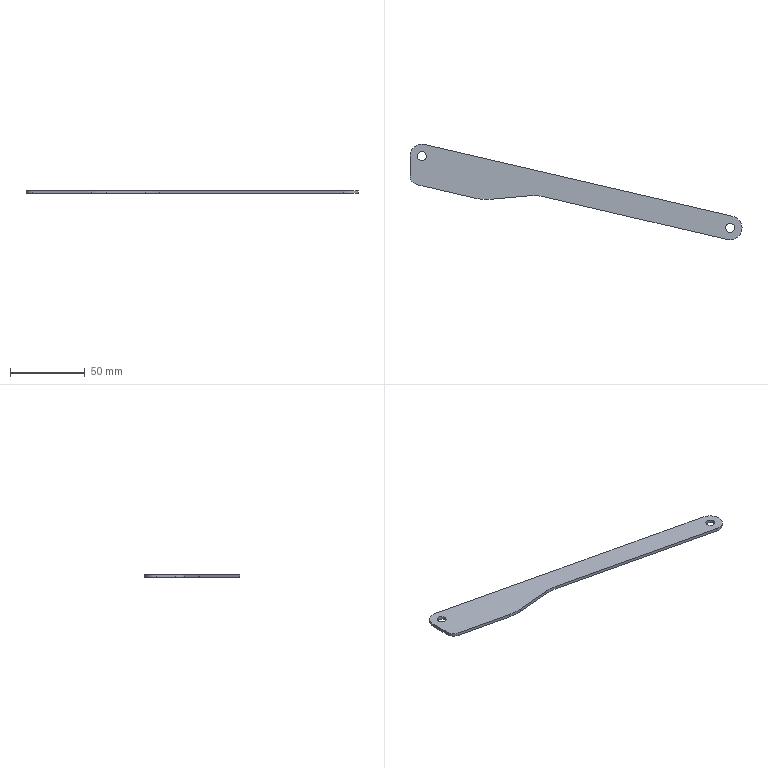Part | STEP file | 1 solid | 17 faces | box 222 x 64 x 2 mm | volume 8617 mm3 | cylinder 10 | plane 7 | commonest cylinder face diameters 6 x4 16 x3 60 x2 12 x1
STEP:
#1=CARTESIAN_POINT('',(0.,0.,0.));
#2=DIRECTION('',(0.,0.,1.));
#3=DIRECTION('',(1.,0.,0.));
#4=AXIS2_PLACEMENT_3D('',#1,#2,#3);
#5=CARTESIAN_POINT('',(115.253,-83.444,2.));
#6=VERTEX_POINT('',#5);
#7=CARTESIAN_POINT('',(125.069,-75.653,2.));
#8=VERTEX_POINT('',#7);
#9=CARTESIAN_POINT('',(117.069,-75.653,2.));
#10=DIRECTION('',(0.,0.,1.));
#11=DIRECTION('',(1.,0.,0.));
#12=AXIS2_PLACEMENT_3D('',#9,#10,#11);
#13=CIRCLE('',#12,8.);
#14=CARTESIAN_POINT('',(117.069,-75.653,2.));
#15=DIRECTION('',(0.,0.,1.));
#16=DIRECTION('',(1.,0.,0.));
#17=AXIS2_PLACEMENT_3D('',#14,#15,#16);
#18=CYLINDRICAL_SURFACE('',#17,8.);
#19=CARTESIAN_POINT('',(0.,0.));
#20=DIRECTION('',(1.,0.));
#21=VECTOR('',#20,1.);
#22=LINE('',#19,#21);
#23=(GEOMETRIC_REPRESENTATION_CONTEXT(2)PARAMETRIC_REPRESENTATION_CONTEXT()REPRESENTATION_CONTEXT('',''));
#24=DEFINITIONAL_REPRESENTATION('',(#22),#23);
#25=PCURVE('',#18,#24);
#26=CARTESIAN_POINT('',(11.579,-52.884,2.));
#27=DIRECTION('',(0.,0.,1.));
#28=DIRECTION('',(1.,0.,0.));
#29=AXIS2_PLACEMENT_3D('',#26,#27,#28);
#30=PLANE('',#29);
#31=CARTESIAN_POINT('',(105.49,-22.769));
#32=DIRECTION('',(1.,0.));
#33=AXIS2_PLACEMENT_2D('',#31,#32);
#34=CIRCLE('',#33,8.);
#35=(GEOMETRIC_REPRESENTATION_CONTEXT(2)PARAMETRIC_REPRESENTATION_CONTEXT()REPRESENTATION_CONTEXT('',''));
#36=DEFINITIONAL_REPRESENTATION('',(#34),#35);
#37=PCURVE('',#30,#36);
#38=SURFACE_CURVE('',#13,(#25,#37),.PCURVE_S1.);
#39=EDGE_CURVE('',#6,#8,#38,.T.);
#40=ORIENTED_EDGE('',*,*,#39,.T.);
#41=CARTESIAN_POINT('',(125.069,-75.653,4.));
#42=VERTEX_POINT('',#41);
#43=CARTESIAN_POINT('',(125.069,-75.653,2.));
#44=DIRECTION('',(0.,0.,1.));
#45=VECTOR('',#44,1.);
#46=LINE('',#43,#45);
#47=CARTESIAN_POINT('',(6.283,0.));
#48=DIRECTION('',(0.,1.));
#49=VECTOR('',#48,1.);
#50=LINE('',#47,#49);
#51=(GEOMETRIC_REPRESENTATION_CONTEXT(2)PARAMETRIC_REPRESENTATION_CONTEXT()REPRESENTATION_CONTEXT('',''));
#52=DEFINITIONAL_REPRESENTATION('',(#50),#51);
#53=PCURVE('',#18,#52);
#54=CARTESIAN_POINT('',(117.069,-75.653,2.));
#55=DIRECTION('',(0.,0.,1.));
#56=DIRECTION('',(1.,0.,0.));
#57=AXIS2_PLACEMENT_3D('',#54,#55,#56);
#58=CYLINDRICAL_SURFACE('',#57,8.);
#59=CARTESIAN_POINT('',(0.,0.));
#60=DIRECTION('',(0.,1.));
#61=VECTOR('',#60,1.);
#62=LINE('',#59,#61);
#63=(GEOMETRIC_REPRESENTATION_CONTEXT(2)PARAMETRIC_REPRESENTATION_CONTEXT()REPRESENTATION_CONTEXT('',''));
#64=DEFINITIONAL_REPRESENTATION('',(#62),#63);
#65=PCURVE('',#58,#64);
#66=SURFACE_CURVE('',#46,(#53,#65),.PCURVE_S1.);
#67=EDGE_CURVE('',#8,#42,#66,.T.);
#68=ORIENTED_EDGE('',*,*,#67,.T.);
#69=CARTESIAN_POINT('',(115.253,-83.444,4.));
#70=VERTEX_POINT('',#69);
#71=CARTESIAN_POINT('',(117.069,-75.653,4.));
#72=DIRECTION('',(0.,0.,-1.));
#73=DIRECTION('',(1.,0.,0.));
#74=AXIS2_PLACEMENT_3D('',#71,#72,#73);
#75=CIRCLE('',#74,8.);
#76=CARTESIAN_POINT('',(6.283,2.));
#77=DIRECTION('',(-1.,0.));
#78=VECTOR('',#77,1.);
#79=LINE('',#76,#78);
#80=(GEOMETRIC_REPRESENTATION_CONTEXT(2)PARAMETRIC_REPRESENTATION_CONTEXT()REPRESENTATION_CONTEXT('',''));
#81=DEFINITIONAL_REPRESENTATION('',(#79),#80);
#82=PCURVE('',#18,#81);
#83=CARTESIAN_POINT('',(11.579,-52.884,4.));
#84=DIRECTION('',(0.,0.,1.));
#85=DIRECTION('',(1.,0.,0.));
#86=AXIS2_PLACEMENT_3D('',#83,#84,#85);
#87=PLANE('',#86);
#88=CARTESIAN_POINT('',(113.49,-22.769));
#89=CARTESIAN_POINT('',(113.49,-36.625));
#90=CARTESIAN_POINT('',(101.49,-29.697));
#91=CARTESIAN_POINT('',(89.49,-22.769));
#92=CARTESIAN_POINT('',(101.49,-15.841));
#93=CARTESIAN_POINT('',(113.49,-8.912));
#94=CARTESIAN_POINT('',(113.49,-22.769));
#95=(BOUNDED_CURVE()B_SPLINE_CURVE(2,(#88,#89,#90,#91,#92,#93,#94),.UNSPECIFIED.,.T.,.F.)B_SPLINE_CURVE_WITH_KNOTS((1,2,2,2,2,1),(-2.094,0.,2.094,4.189,6.283,8.378),.UNSPECIFIED.)CURVE()GEOMETRIC_REPRESENTATION_ITEM()RATIONAL_B_SPLINE_CURVE((1.,0.5,1.,0.5,1.,0.5,1.))REPRESENTATION_ITEM(''));
#96=(GEOMETRIC_REPRESENTATION_CONTEXT(2)PARAMETRIC_REPRESENTATION_CONTEXT()REPRESENTATION_CONTEXT('',''));
#97=DEFINITIONAL_REPRESENTATION('',(#95),#96);
#98=PCURVE('',#87,#97);
#99=SURFACE_CURVE('',#75,(#82,#98),.PCURVE_S1.);
#100=EDGE_CURVE('',#42,#70,#99,.T.);
#101=ORIENTED_EDGE('',*,*,#100,.T.);
#102=CARTESIAN_POINT('',(115.253,-83.444,2.));
#103=DIRECTION('',(0.,0.,-1.));
#104=VECTOR('',#103,1.);
#105=LINE('',#102,#104);
#106=CARTESIAN_POINT('',(4.483,0.));
#107=DIRECTION('',(0.,-1.));
#108=VECTOR('',#107,1.);
#109=LINE('',#106,#108);
#110=(GEOMETRIC_REPRESENTATION_CONTEXT(2)PARAMETRIC_REPRESENTATION_CONTEXT()REPRESENTATION_CONTEXT('',''));
#111=DEFINITIONAL_REPRESENTATION('',(#109),#110);
#112=PCURVE('',#18,#111);
#113=CARTESIAN_POINT('',(-7.662,-54.804,2.));
#114=DIRECTION('',(-0.2269,-0.9739,0.));
#115=DIRECTION('',(0.9739,-0.2269,0.));
#116=AXIS2_PLACEMENT_3D('',#113,#114,#115);
#117=PLANE('',#116);
#118=CARTESIAN_POINT('',(126.208,0.));
#119=DIRECTION('',(0.,-1.));
#120=VECTOR('',#119,1.);
#121=LINE('',#118,#120);
#122=(GEOMETRIC_REPRESENTATION_CONTEXT(2)PARAMETRIC_REPRESENTATION_CONTEXT()REPRESENTATION_CONTEXT('',''));
#123=DEFINITIONAL_REPRESENTATION('',(#121),#122);
#124=PCURVE('',#117,#123);
#125=SURFACE_CURVE('',#105,(#112,#124),.PCURVE_S1.);
#126=EDGE_CURVE('',#70,#6,#125,.T.);
#127=ORIENTED_EDGE('',*,*,#126,.T.);
#128=EDGE_LOOP('',(#40,#68,#101,#127));
#129=FACE_BOUND('',#128,.T.);
#130=ADVANCED_FACE('',(#129),#18,.T.);
#131=CARTESIAN_POINT('',(120.069,-75.653,2.));
#132=VERTEX_POINT('',#131);
#133=CARTESIAN_POINT('',(120.069,-75.653,4.));
#134=VERTEX_POINT('',#133);
#135=CARTESIAN_POINT('',(120.069,-75.653,2.));
#136=DIRECTION('',(0.,0.,1.));
#137=VECTOR('',#136,1.);
#138=LINE('',#135,#137);
#139=CARTESIAN_POINT('',(117.069,-75.653,2.));
#140=DIRECTION('',(0.,0.,1.));
#141=DIRECTION('',(1.,0.,0.));
#142=AXIS2_PLACEMENT_3D('',#139,#140,#141);
#143=CYLINDRICAL_SURFACE('',#142,3.);
#144=CARTESIAN_POINT('',(6.283,0.));
#145=DIRECTION('',(0.,1.));
#146=VECTOR('',#145,1.);
#147=LINE('',#144,#146);
#148=(GEOMETRIC_REPRESENTATION_CONTEXT(2)PARAMETRIC_REPRESENTATION_CONTEXT()REPRESENTATION_CONTEXT('',''));
#149=DEFINITIONAL_REPRESENTATION('',(#147),#148);
#150=PCURVE('',#143,#149);
#151=CARTESIAN_POINT('',(117.069,-75.653,2.));
#152=DIRECTION('',(0.,0.,1.));
#153=DIRECTION('',(1.,0.,0.));
#154=AXIS2_PLACEMENT_3D('',#151,#152,#153);
#155=CYLINDRICAL_SURFACE('',#154,3.);
#156=CARTESIAN_POINT('',(0.,0.));
#157=DIRECTION('',(0.,1.));
#158=VECTOR('',#157,1.);
#159=LINE('',#156,#158);
#160=(GEOMETRIC_REPRESENTATION_CONTEXT(2)PARAMETRIC_REPRESENTATION_CONTEXT()REPRESENTATION_CONTEXT('',''));
#161=DEFINITIONAL_REPRESENTATION('',(#159),#160);
#162=PCURVE('',#155,#161);
#163=SURFACE_CURVE('',#138,(#150,#162),.PCURVE_S1.);
#164=EDGE_CURVE('',#132,#134,#163,.T.);
#165=ORIENTED_EDGE('',*,*,#164,.T.);
#166=CARTESIAN_POINT('',(114.069,-75.653,4.));
#167=VERTEX_POINT('',#166);
#168=CARTESIAN_POINT('',(117.069,-75.653,4.));
#169=DIRECTION('',(0.,0.,-1.));
#170=DIRECTION('',(1.,0.,0.));
#171=AXIS2_PLACEMENT_3D('',#168,#169,#170);
#172=CIRCLE('',#171,3.);
#173=CARTESIAN_POINT('',(6.283,2.));
#174=DIRECTION('',(-1.,0.));
#175=VECTOR('',#174,1.);
#176=LINE('',#173,#175);
#177=(GEOMETRIC_REPRESENTATION_CONTEXT(2)PARAMETRIC_REPRESENTATION_CONTEXT()REPRESENTATION_CONTEXT('',''));
#178=DEFINITIONAL_REPRESENTATION('',(#176),#177);
#179=PCURVE('',#143,#178);
#180=CARTESIAN_POINT('',(108.49,-22.769));
#181=CARTESIAN_POINT('',(108.49,-27.965));
#182=CARTESIAN_POINT('',(103.99,-25.367));
#183=CARTESIAN_POINT('',(99.49,-22.769));
#184=CARTESIAN_POINT('',(103.99,-20.171));
#185=CARTESIAN_POINT('',(108.49,-17.573));
#186=CARTESIAN_POINT('',(108.49,-22.769));
#187=(BOUNDED_CURVE()B_SPLINE_CURVE(2,(#180,#181,#182,#183,#184,#185,#186),.UNSPECIFIED.,.T.,.F.)B_SPLINE_CURVE_WITH_KNOTS((1,2,2,2,2,1),(-2.094,0.,2.094,4.189,6.283,8.378),.UNSPECIFIED.)CURVE()GEOMETRIC_REPRESENTATION_ITEM()RATIONAL_B_SPLINE_CURVE((1.,0.5,1.,0.5,1.,0.5,1.))REPRESENTATION_ITEM(''));
#188=(GEOMETRIC_REPRESENTATION_CONTEXT(2)PARAMETRIC_REPRESENTATION_CONTEXT()REPRESENTATION_CONTEXT('',''));
#189=DEFINITIONAL_REPRESENTATION('',(#187),#188);
#190=PCURVE('',#87,#189);
#191=SURFACE_CURVE('',#172,(#179,#190),.PCURVE_S1.);
#192=EDGE_CURVE('',#134,#167,#191,.T.);
#193=ORIENTED_EDGE('',*,*,#192,.T.);
#194=CARTESIAN_POINT('',(114.069,-75.653,2.));
#195=VERTEX_POINT('',#194);
#196=CARTESIAN_POINT('',(114.069,-75.653,2.));
#197=DIRECTION('',(0.,0.,1.));
#198=VECTOR('',#197,1.);
#199=LINE('',#196,#198);
#200=CARTESIAN_POINT('',(3.142,0.));
#201=DIRECTION('',(0.,1.));
#202=VECTOR('',#201,1.);
#203=LINE('',#200,#202);
#204=(GEOMETRIC_REPRESENTATION_CONTEXT(2)PARAMETRIC_REPRESENTATION_CONTEXT()REPRESENTATION_CONTEXT('',''));
#205=DEFINITIONAL_REPRESENTATION('',(#203),#204);
#206=PCURVE('',#143,#205);
#207=CARTESIAN_POINT('',(3.142,0.));
#208=DIRECTION('',(0.,1.));
#209=VECTOR('',#208,1.);
#210=LINE('',#207,#209);
#211=(GEOMETRIC_REPRESENTATION_CONTEXT(2)PARAMETRIC_REPRESENTATION_CONTEXT()REPRESENTATION_CONTEXT('',''));
#212=DEFINITIONAL_REPRESENTATION('',(#210),#211);
#213=PCURVE('',#155,#212);
#214=SURFACE_CURVE('',#199,(#206,#213),.PCURVE_S1.);
#215=EDGE_CURVE('',#195,#167,#214,.T.);
#216=ORIENTED_EDGE('',*,*,#215,.F.);
#217=CARTESIAN_POINT('',(117.069,-75.653,2.));
#218=DIRECTION('',(0.,0.,-1.));
#219=DIRECTION('',(1.,0.,0.));
#220=AXIS2_PLACEMENT_3D('',#217,#218,#219);
#221=CIRCLE('',#220,3.);
#222=CARTESIAN_POINT('',(6.283,0.));
#223=DIRECTION('',(-1.,0.));
#224=VECTOR('',#223,1.);
#225=LINE('',#222,#224);
#226=(GEOMETRIC_REPRESENTATION_CONTEXT(2)PARAMETRIC_REPRESENTATION_CONTEXT()REPRESENTATION_CONTEXT('',''));
#227=DEFINITIONAL_REPRESENTATION('',(#225),#226);
#228=PCURVE('',#143,#227);
#229=CARTESIAN_POINT('',(108.49,-22.769));
#230=CARTESIAN_POINT('',(108.49,-27.965));
#231=CARTESIAN_POINT('',(103.99,-25.367));
#232=CARTESIAN_POINT('',(99.49,-22.769));
#233=CARTESIAN_POINT('',(103.99,-20.171));
#234=CARTESIAN_POINT('',(108.49,-17.573));
#235=CARTESIAN_POINT('',(108.49,-22.769));
#236=(BOUNDED_CURVE()B_SPLINE_CURVE(2,(#229,#230,#231,#232,#233,#234,#235),.UNSPECIFIED.,.T.,.F.)B_SPLINE_CURVE_WITH_KNOTS((1,2,2,2,2,1),(-2.094,0.,2.094,4.189,6.283,8.378),.UNSPECIFIED.)CURVE()GEOMETRIC_REPRESENTATION_ITEM()RATIONAL_B_SPLINE_CURVE((1.,0.5,1.,0.5,1.,0.5,1.))REPRESENTATION_ITEM(''));
#237=(GEOMETRIC_REPRESENTATION_CONTEXT(2)PARAMETRIC_REPRESENTATION_CONTEXT()REPRESENTATION_CONTEXT('',''));
#238=DEFINITIONAL_REPRESENTATION('',(#236),#237);
#239=PCURVE('',#30,#238);
#240=SURFACE_CURVE('',#221,(#228,#239),.PCURVE_S1.);
#241=EDGE_CURVE('',#132,#195,#240,.T.);
#242=ORIENTED_EDGE('',*,*,#241,.F.);
#243=EDGE_LOOP('',(#165,#193,#216,#242));
#244=FACE_BOUND('',#243,.F.);
#245=ADVANCED_FACE('',(#244),#143,.F.);
#246=CARTESIAN_POINT('',(-85.931,-27.653,2.));
#247=VERTEX_POINT('',#246);
#248=CARTESIAN_POINT('',(-85.931,-27.653,4.));
#249=VERTEX_POINT('',#248);
#250=CARTESIAN_POINT('',(-85.931,-27.653,2.));
#251=DIRECTION('',(0.,0.,1.));
#252=VECTOR('',#251,1.);
#253=LINE('',#250,#252);
#254=CARTESIAN_POINT('',(-88.931,-27.653,2.));
#255=DIRECTION('',(0.,0.,1.));
#256=DIRECTION('',(1.,0.,0.));
#257=AXIS2_PLACEMENT_3D('',#254,#255,#256);
#258=CYLINDRICAL_SURFACE('',#257,3.);
#259=CARTESIAN_POINT('',(6.283,0.));
#260=DIRECTION('',(0.,1.));
#261=VECTOR('',#260,1.);
#262=LINE('',#259,#261);
#263=(GEOMETRIC_REPRESENTATION_CONTEXT(2)PARAMETRIC_REPRESENTATION_CONTEXT()REPRESENTATION_CONTEXT('',''));
#264=DEFINITIONAL_REPRESENTATION('',(#262),#263);
#265=PCURVE('',#258,#264);
#266=CARTESIAN_POINT('',(-88.931,-27.653,2.));
#267=DIRECTION('',(0.,0.,1.));
#268=DIRECTION('',(1.,0.,0.));
#269=AXIS2_PLACEMENT_3D('',#266,#267,#268);
#270=CYLINDRICAL_SURFACE('',#269,3.);
#271=CARTESIAN_POINT('',(0.,0.));
#272=DIRECTION('',(0.,1.));
#273=VECTOR('',#272,1.);
#274=LINE('',#271,#273);
#275=(GEOMETRIC_REPRESENTATION_CONTEXT(2)PARAMETRIC_REPRESENTATION_CONTEXT()REPRESENTATION_CONTEXT('',''));
#276=DEFINITIONAL_REPRESENTATION('',(#274),#275);
#277=PCURVE('',#270,#276);
#278=SURFACE_CURVE('',#253,(#265,#277),.PCURVE_S1.);
#279=EDGE_CURVE('',#247,#249,#278,.T.);
#280=ORIENTED_EDGE('',*,*,#279,.T.);
#281=CARTESIAN_POINT('',(-91.931,-27.653,4.));
#282=VERTEX_POINT('',#281);
#283=CARTESIAN_POINT('',(-88.931,-27.653,4.));
#284=DIRECTION('',(0.,0.,-1.));
#285=DIRECTION('',(1.,0.,0.));
#286=AXIS2_PLACEMENT_3D('',#283,#284,#285);
#287=CIRCLE('',#286,3.);
#288=CARTESIAN_POINT('',(6.283,2.));
#289=DIRECTION('',(-1.,0.));
#290=VECTOR('',#289,1.);
#291=LINE('',#288,#290);
#292=(GEOMETRIC_REPRESENTATION_CONTEXT(2)PARAMETRIC_REPRESENTATION_CONTEXT()REPRESENTATION_CONTEXT('',''));
#293=DEFINITIONAL_REPRESENTATION('',(#291),#292);
#294=PCURVE('',#258,#293);
#295=CARTESIAN_POINT('',(-97.51,25.231));
#296=CARTESIAN_POINT('',(-97.51,20.035));
#297=CARTESIAN_POINT('',(-102.01,22.633));
#298=CARTESIAN_POINT('',(-106.51,25.231));
#299=CARTESIAN_POINT('',(-102.01,27.829));
#300=CARTESIAN_POINT('',(-97.51,30.427));
#301=CARTESIAN_POINT('',(-97.51,25.231));
#302=(BOUNDED_CURVE()B_SPLINE_CURVE(2,(#295,#296,#297,#298,#299,#300,#301),.UNSPECIFIED.,.T.,.F.)B_SPLINE_CURVE_WITH_KNOTS((1,2,2,2,2,1),(-2.094,0.,2.094,4.189,6.283,8.378),.UNSPECIFIED.)CURVE()GEOMETRIC_REPRESENTATION_ITEM()RATIONAL_B_SPLINE_CURVE((1.,0.5,1.,0.5,1.,0.5,1.))REPRESENTATION_ITEM(''));
#303=(GEOMETRIC_REPRESENTATION_CONTEXT(2)PARAMETRIC_REPRESENTATION_CONTEXT()REPRESENTATION_CONTEXT('',''));
#304=DEFINITIONAL_REPRESENTATION('',(#302),#303);
#305=PCURVE('',#87,#304);
#306=SURFACE_CURVE('',#287,(#294,#305),.PCURVE_S1.);
#307=EDGE_CURVE('',#249,#282,#306,.T.);
#308=ORIENTED_EDGE('',*,*,#307,.T.);
#309=CARTESIAN_POINT('',(-91.931,-27.653,2.));
#310=VERTEX_POINT('',#309);
#311=CARTESIAN_POINT('',(-91.931,-27.653,2.));
#312=DIRECTION('',(0.,0.,1.));
#313=VECTOR('',#312,1.);
#314=LINE('',#311,#313);
#315=CARTESIAN_POINT('',(3.142,0.));
#316=DIRECTION('',(0.,1.));
#317=VECTOR('',#316,1.);
#318=LINE('',#315,#317);
#319=(GEOMETRIC_REPRESENTATION_CONTEXT(2)PARAMETRIC_REPRESENTATION_CONTEXT()REPRESENTATION_CONTEXT('',''));
#320=DEFINITIONAL_REPRESENTATION('',(#318),#319);
#321=PCURVE('',#258,#320);
#322=CARTESIAN_POINT('',(3.142,0.));
#323=DIRECTION('',(0.,1.));
#324=VECTOR('',#323,1.);
#325=LINE('',#322,#324);
#326=(GEOMETRIC_REPRESENTATION_CONTEXT(2)PARAMETRIC_REPRESENTATION_CONTEXT()REPRESENTATION_CONTEXT('',''));
#327=DEFINITIONAL_REPRESENTATION('',(#325),#326);
#328=PCURVE('',#270,#327);
#329=SURFACE_CURVE('',#314,(#321,#328),.PCURVE_S1.);
#330=EDGE_CURVE('',#310,#282,#329,.T.);
#331=ORIENTED_EDGE('',*,*,#330,.F.);
#332=CARTESIAN_POINT('',(-88.931,-27.653,2.));
#333=DIRECTION('',(0.,0.,-1.));
#334=DIRECTION('',(1.,0.,0.));
#335=AXIS2_PLACEMENT_3D('',#332,#333,#334);
#336=CIRCLE('',#335,3.);
#337=CARTESIAN_POINT('',(6.283,0.));
#338=DIRECTION('',(-1.,0.));
#339=VECTOR('',#338,1.);
#340=LINE('',#337,#339);
#341=(GEOMETRIC_REPRESENTATION_CONTEXT(2)PARAMETRIC_REPRESENTATION_CONTEXT()REPRESENTATION_CONTEXT('',''));
#342=DEFINITIONAL_REPRESENTATION('',(#340),#341);
#343=PCURVE('',#258,#342);
#344=CARTESIAN_POINT('',(-97.51,25.231));
#345=CARTESIAN_POINT('',(-97.51,20.035));
#346=CARTESIAN_POINT('',(-102.01,22.633));
#347=CARTESIAN_POINT('',(-106.51,25.231));
#348=CARTESIAN_POINT('',(-102.01,27.829));
#349=CARTESIAN_POINT('',(-97.51,30.427));
#350=CARTESIAN_POINT('',(-97.51,25.231));
#351=(BOUNDED_CURVE()B_SPLINE_CURVE(2,(#344,#345,#346,#347,#348,#349,#350),.UNSPECIFIED.,.T.,.F.)B_SPLINE_CURVE_WITH_KNOTS((1,2,2,2,2,1),(-2.094,0.,2.094,4.189,6.283,8.378),.UNSPECIFIED.)CURVE()GEOMETRIC_REPRESENTATION_ITEM()RATIONAL_B_SPLINE_CURVE((1.,0.5,1.,0.5,1.,0.5,1.))REPRESENTATION_ITEM(''));
#352=(GEOMETRIC_REPRESENTATION_CONTEXT(2)PARAMETRIC_REPRESENTATION_CONTEXT()REPRESENTATION_CONTEXT('',''));
#353=DEFINITIONAL_REPRESENTATION('',(#351),#352);
#354=PCURVE('',#30,#353);
#355=SURFACE_CURVE('',#336,(#343,#354),.PCURVE_S1.);
#356=EDGE_CURVE('',#247,#310,#355,.T.);
#357=ORIENTED_EDGE('',*,*,#356,.F.);
#358=EDGE_LOOP('',(#280,#308,#331,#357));
#359=FACE_BOUND('',#358,.F.);
#360=ADVANCED_FACE('',(#359),#258,.F.);
#361=ORIENTED_EDGE('',*,*,#39,.F.);
#362=CARTESIAN_POINT('',(-7.662,-54.804,2.));
#363=VERTEX_POINT('',#362);
#364=CARTESIAN_POINT('',(-7.662,-54.804,2.));
#365=DIRECTION('',(0.9739,-0.2269,0.));
#366=VECTOR('',#365,1.);
#367=LINE('',#364,#366);
#368=CARTESIAN_POINT('',(-19.242,-1.919));
#369=DIRECTION('',(0.9739,-0.2269));
#370=VECTOR('',#369,1.);
#371=LINE('',#368,#370);
#372=(GEOMETRIC_REPRESENTATION_CONTEXT(2)PARAMETRIC_REPRESENTATION_CONTEXT()REPRESENTATION_CONTEXT('',''));
#373=DEFINITIONAL_REPRESENTATION('',(#371),#372);
#374=PCURVE('',#30,#373);
#375=CARTESIAN_POINT('',(0.,0.));
#376=DIRECTION('',(1.,0.));
#377=VECTOR('',#376,1.);
#378=LINE('',#375,#377);
#379=(GEOMETRIC_REPRESENTATION_CONTEXT(2)PARAMETRIC_REPRESENTATION_CONTEXT()REPRESENTATION_CONTEXT('',''));
#380=DEFINITIONAL_REPRESENTATION('',(#378),#379);
#381=PCURVE('',#117,#380);
#382=SURFACE_CURVE('',#367,(#374,#381),.PCURVE_S1.);
#383=EDGE_CURVE('',#363,#6,#382,.T.);
#384=ORIENTED_EDGE('',*,*,#383,.F.);
#385=CARTESIAN_POINT('',(-17.217,-54.147,2.));
#386=VERTEX_POINT('',#385);
#387=CARTESIAN_POINT('',(-14.47,-84.021,2.));
#388=DIRECTION('',(0.,0.,-1.));
#389=DIRECTION('',(1.,0.,0.));
#390=AXIS2_PLACEMENT_3D('',#387,#388,#389);
#391=CIRCLE('',#390,30.);
#392=CARTESIAN_POINT('',(3.95,-31.137));
#393=CARTESIAN_POINT('',(3.95,-83.098));
#394=CARTESIAN_POINT('',(-41.05,-57.118));
#395=CARTESIAN_POINT('',(-86.05,-31.137));
#396=CARTESIAN_POINT('',(-41.05,-5.156));
#397=CARTESIAN_POINT('',(3.95,20.825));
#398=CARTESIAN_POINT('',(3.95,-31.137));
#399=(BOUNDED_CURVE()B_SPLINE_CURVE(2,(#392,#393,#394,#395,#396,#397,#398),.UNSPECIFIED.,.T.,.F.)B_SPLINE_CURVE_WITH_KNOTS((1,2,2,2,2,1),(-2.094,0.,2.094,4.189,6.283,8.378),.UNSPECIFIED.)CURVE()GEOMETRIC_REPRESENTATION_ITEM()RATIONAL_B_SPLINE_CURVE((1.,0.5,1.,0.5,1.,0.5,1.))REPRESENTATION_ITEM(''));
#400=(GEOMETRIC_REPRESENTATION_CONTEXT(2)PARAMETRIC_REPRESENTATION_CONTEXT()REPRESENTATION_CONTEXT('',''));
#401=DEFINITIONAL_REPRESENTATION('',(#399),#400);
#402=PCURVE('',#30,#401);
#403=CARTESIAN_POINT('',(-14.47,-84.021,2.));
#404=DIRECTION('',(0.,0.,1.));
#405=DIRECTION('',(1.,0.,0.));
#406=AXIS2_PLACEMENT_3D('',#403,#404,#405);
#407=CYLINDRICAL_SURFACE('',#406,30.);
#408=CARTESIAN_POINT('',(6.283,0.));
#409=DIRECTION('',(-1.,0.));
#410=VECTOR('',#409,1.);
#411=LINE('',#408,#410);
#412=(GEOMETRIC_REPRESENTATION_CONTEXT(2)PARAMETRIC_REPRESENTATION_CONTEXT()REPRESENTATION_CONTEXT('',''));
#413=DEFINITIONAL_REPRESENTATION('',(#411),#412);
#414=PCURVE('',#407,#413);
#415=SURFACE_CURVE('',#391,(#402,#414),.PCURVE_S1.);
#416=EDGE_CURVE('',#386,#363,#415,.T.);
#417=ORIENTED_EDGE('',*,*,#416,.F.);
#418=CARTESIAN_POINT('',(-43.405,-56.555,2.));
#419=VERTEX_POINT('',#418);
#420=CARTESIAN_POINT('',(-43.405,-56.555,2.));
#421=DIRECTION('',(0.9958,0.09157,0.));
#422=VECTOR('',#421,1.);
#423=LINE('',#420,#422);
#424=CARTESIAN_POINT('',(-54.984,-3.671));
#425=DIRECTION('',(0.9958,0.09157));
#426=VECTOR('',#425,1.);
#427=LINE('',#424,#426);
#428=(GEOMETRIC_REPRESENTATION_CONTEXT(2)PARAMETRIC_REPRESENTATION_CONTEXT()REPRESENTATION_CONTEXT('',''));
#429=DEFINITIONAL_REPRESENTATION('',(#427),#428);
#430=PCURVE('',#30,#429);
#431=CARTESIAN_POINT('',(-43.405,-56.555,2.));
#432=DIRECTION('',(0.09157,-0.9958,0.));
#433=DIRECTION('',(0.9958,0.09157,0.));
#434=AXIS2_PLACEMENT_3D('',#431,#432,#433);
#435=PLANE('',#434);
#436=CARTESIAN_POINT('',(0.,0.));
#437=DIRECTION('',(1.,0.));
#438=VECTOR('',#437,1.);
#439=LINE('',#436,#438);
#440=(GEOMETRIC_REPRESENTATION_CONTEXT(2)PARAMETRIC_REPRESENTATION_CONTEXT()REPRESENTATION_CONTEXT('',''));
#441=DEFINITIONAL_REPRESENTATION('',(#439),#440);
#442=PCURVE('',#435,#441);
#443=SURFACE_CURVE('',#423,(#430,#442),.PCURVE_S1.);
#444=EDGE_CURVE('',#419,#386,#443,.T.);
#445=ORIENTED_EDGE('',*,*,#444,.F.);
#446=CARTESIAN_POINT('',(-52.96,-55.899,2.));
#447=VERTEX_POINT('',#446);
#448=CARTESIAN_POINT('',(-46.152,-26.681,2.));
#449=DIRECTION('',(0.,0.,1.));
#450=DIRECTION('',(1.,0.,0.));
#451=AXIS2_PLACEMENT_3D('',#448,#449,#450);
#452=CIRCLE('',#451,30.);
#453=CARTESIAN_POINT('',(-57.731,26.203));
#454=DIRECTION('',(1.,0.));
#455=AXIS2_PLACEMENT_2D('',#453,#454);
#456=CIRCLE('',#455,30.);
#457=(GEOMETRIC_REPRESENTATION_CONTEXT(2)PARAMETRIC_REPRESENTATION_CONTEXT()REPRESENTATION_CONTEXT('',''));
#458=DEFINITIONAL_REPRESENTATION('',(#456),#457);
#459=PCURVE('',#30,#458);
#460=CARTESIAN_POINT('',(-46.152,-26.681,2.));
#461=DIRECTION('',(0.,0.,1.));
#462=DIRECTION('',(1.,0.,0.));
#463=AXIS2_PLACEMENT_3D('',#460,#461,#462);
#464=CYLINDRICAL_SURFACE('',#463,30.);
#465=CARTESIAN_POINT('',(0.,0.));
#466=DIRECTION('',(1.,0.));
#467=VECTOR('',#466,1.);
#468=LINE('',#465,#467);
#469=(GEOMETRIC_REPRESENTATION_CONTEXT(2)PARAMETRIC_REPRESENTATION_CONTEXT()REPRESENTATION_CONTEXT('',''));
#470=DEFINITIONAL_REPRESENTATION('',(#468),#469);
#471=PCURVE('',#464,#470);
#472=SURFACE_CURVE('',#452,(#459,#471),.PCURVE_S1.);
#473=EDGE_CURVE('',#447,#419,#472,.T.);
#474=ORIENTED_EDGE('',*,*,#473,.F.);
#475=CARTESIAN_POINT('',(-92.293,-46.734,2.));
#476=VERTEX_POINT('',#475);
#477=CARTESIAN_POINT('',(-92.293,-46.734,2.));
#478=DIRECTION('',(0.9739,-0.2269,0.));
#479=VECTOR('',#478,1.);
#480=LINE('',#477,#479);
#481=CARTESIAN_POINT('',(-103.872,6.15));
#482=DIRECTION('',(0.9739,-0.2269));
#483=VECTOR('',#482,1.);
#484=LINE('',#481,#483);
#485=(GEOMETRIC_REPRESENTATION_CONTEXT(2)PARAMETRIC_REPRESENTATION_CONTEXT()REPRESENTATION_CONTEXT('',''));
#486=DEFINITIONAL_REPRESENTATION('',(#484),#485);
#487=PCURVE('',#30,#486);
#488=CARTESIAN_POINT('',(-92.293,-46.734,2.));
#489=DIRECTION('',(-0.2269,-0.9739,0.));
#490=DIRECTION('',(0.9739,-0.2269,0.));
#491=AXIS2_PLACEMENT_3D('',#488,#489,#490);
#492=PLANE('',#491);
#493=CARTESIAN_POINT('',(0.,0.));
#494=DIRECTION('',(1.,0.));
#495=VECTOR('',#494,1.);
#496=LINE('',#493,#495);
#497=(GEOMETRIC_REPRESENTATION_CONTEXT(2)PARAMETRIC_REPRESENTATION_CONTEXT()REPRESENTATION_CONTEXT('',''));
#498=DEFINITIONAL_REPRESENTATION('',(#496),#497);
#499=PCURVE('',#492,#498);
#500=SURFACE_CURVE('',#480,(#487,#499),.PCURVE_S1.);
#501=EDGE_CURVE('',#476,#447,#500,.T.);
#502=ORIENTED_EDGE('',*,*,#501,.F.);
#503=CARTESIAN_POINT('',(-96.931,-40.89,2.));
#504=VERTEX_POINT('',#503);
#505=CARTESIAN_POINT('',(-90.931,-40.89,2.));
#506=DIRECTION('',(0.,0.,1.));
#507=DIRECTION('',(1.,0.,0.));
#508=AXIS2_PLACEMENT_3D('',#505,#506,#507);
#509=CIRCLE('',#508,6.);
#510=CARTESIAN_POINT('',(-102.51,11.994));
#511=DIRECTION('',(1.,0.));
#512=AXIS2_PLACEMENT_2D('',#510,#511);
#513=CIRCLE('',#512,6.);
#514=(GEOMETRIC_REPRESENTATION_CONTEXT(2)PARAMETRIC_REPRESENTATION_CONTEXT()REPRESENTATION_CONTEXT('',''));
#515=DEFINITIONAL_REPRESENTATION('',(#513),#514);
#516=PCURVE('',#30,#515);
#517=CARTESIAN_POINT('',(-90.931,-40.89,2.));
#518=DIRECTION('',(0.,0.,1.));
#519=DIRECTION('',(1.,0.,0.));
#520=AXIS2_PLACEMENT_3D('',#517,#518,#519);
#521=CYLINDRICAL_SURFACE('',#520,6.);
#522=CARTESIAN_POINT('',(0.,0.));
#523=DIRECTION('',(1.,0.));
#524=VECTOR('',#523,1.);
#525=LINE('',#522,#524);
#526=(GEOMETRIC_REPRESENTATION_CONTEXT(2)PARAMETRIC_REPRESENTATION_CONTEXT()REPRESENTATION_CONTEXT('',''));
#527=DEFINITIONAL_REPRESENTATION('',(#525),#526);
#528=PCURVE('',#521,#527);
#529=SURFACE_CURVE('',#509,(#516,#528),.PCURVE_S1.);
#530=EDGE_CURVE('',#504,#476,#529,.T.);
#531=ORIENTED_EDGE('',*,*,#530,.F.);
#532=CARTESIAN_POINT('',(-96.931,-27.653,2.));
#533=VERTEX_POINT('',#532);
#534=CARTESIAN_POINT('',(-96.931,-52.884,2.));
#535=DIRECTION('',(0.,-1.,0.));
#536=VECTOR('',#535,1.);
#537=LINE('',#534,#536);
#538=CARTESIAN_POINT('',(-108.51,0.));
#539=DIRECTION('',(0.,-1.));
#540=VECTOR('',#539,1.);
#541=LINE('',#538,#540);
#542=(GEOMETRIC_REPRESENTATION_CONTEXT(2)PARAMETRIC_REPRESENTATION_CONTEXT()REPRESENTATION_CONTEXT('',''));
#543=DEFINITIONAL_REPRESENTATION('',(#541),#542);
#544=PCURVE('',#30,#543);
#545=CARTESIAN_POINT('',(-96.931,-27.653,2.));
#546=DIRECTION('',(-1.,0.,0.));
#547=DIRECTION('',(0.,-1.,0.));
#548=AXIS2_PLACEMENT_3D('',#545,#546,#547);
#549=PLANE('',#548);
#550=CARTESIAN_POINT('',(25.231,0.));
#551=DIRECTION('',(1.,0.));
#552=VECTOR('',#551,1.);
#553=LINE('',#550,#552);
#554=(GEOMETRIC_REPRESENTATION_CONTEXT(2)PARAMETRIC_REPRESENTATION_CONTEXT()REPRESENTATION_CONTEXT('',''));
#555=DEFINITIONAL_REPRESENTATION('',(#553),#554);
#556=PCURVE('',#549,#555);
#557=SURFACE_CURVE('',#537,(#544,#556),.PCURVE_S1.);
#558=EDGE_CURVE('',#533,#504,#557,.T.);
#559=ORIENTED_EDGE('',*,*,#558,.F.);
#560=CARTESIAN_POINT('',(-87.116,-19.862,2.));
#561=VERTEX_POINT('',#560);
#562=CARTESIAN_POINT('',(-88.931,-27.653,2.));
#563=DIRECTION('',(0.,0.,1.));
#564=DIRECTION('',(1.,0.,0.));
#565=AXIS2_PLACEMENT_3D('',#562,#563,#564);
#566=CIRCLE('',#565,8.);
#567=CARTESIAN_POINT('',(-100.51,25.231));
#568=DIRECTION('',(1.,0.));
#569=AXIS2_PLACEMENT_2D('',#567,#568);
#570=CIRCLE('',#569,8.);
#571=(GEOMETRIC_REPRESENTATION_CONTEXT(2)PARAMETRIC_REPRESENTATION_CONTEXT()REPRESENTATION_CONTEXT('',''));
#572=DEFINITIONAL_REPRESENTATION('',(#570),#571);
#573=PCURVE('',#30,#572);
#574=CARTESIAN_POINT('',(-88.931,-27.653,2.));
#575=DIRECTION('',(0.,0.,1.));
#576=DIRECTION('',(1.,0.,0.));
#577=AXIS2_PLACEMENT_3D('',#574,#575,#576);
#578=CYLINDRICAL_SURFACE('',#577,8.);
#579=CARTESIAN_POINT('',(0.,0.));
#580=DIRECTION('',(1.,0.));
#581=VECTOR('',#580,1.);
#582=LINE('',#579,#581);
#583=(GEOMETRIC_REPRESENTATION_CONTEXT(2)PARAMETRIC_REPRESENTATION_CONTEXT()REPRESENTATION_CONTEXT('',''));
#584=DEFINITIONAL_REPRESENTATION('',(#582),#583);
#585=PCURVE('',#578,#584);
#586=SURFACE_CURVE('',#566,(#573,#585),.PCURVE_S1.);
#587=EDGE_CURVE('',#561,#533,#586,.T.);
#588=ORIENTED_EDGE('',*,*,#587,.F.);
#589=CARTESIAN_POINT('',(118.884,-67.862,2.));
#590=VERTEX_POINT('',#589);
#591=CARTESIAN_POINT('',(118.884,-67.862,2.));
#592=DIRECTION('',(-0.9739,0.2269,0.));
#593=VECTOR('',#592,1.);
#594=LINE('',#591,#593);
#595=CARTESIAN_POINT('',(107.305,-14.977));
#596=DIRECTION('',(-0.9739,0.2269));
#597=VECTOR('',#596,1.);
#598=LINE('',#595,#597);
#599=(GEOMETRIC_REPRESENTATION_CONTEXT(2)PARAMETRIC_REPRESENTATION_CONTEXT()REPRESENTATION_CONTEXT('',''));
#600=DEFINITIONAL_REPRESENTATION('',(#598),#599);
#601=PCURVE('',#30,#600);
#602=CARTESIAN_POINT('',(118.884,-67.862,2.));
#603=DIRECTION('',(0.2269,0.9739,0.));
#604=DIRECTION('',(-0.9739,0.2269,0.));
#605=AXIS2_PLACEMENT_3D('',#602,#603,#604);
#606=PLANE('',#605);
#607=CARTESIAN_POINT('',(0.,0.));
#608=DIRECTION('',(1.,0.));
#609=VECTOR('',#608,1.);
#610=LINE('',#607,#609);
#611=(GEOMETRIC_REPRESENTATION_CONTEXT(2)PARAMETRIC_REPRESENTATION_CONTEXT()REPRESENTATION_CONTEXT('',''));
#612=DEFINITIONAL_REPRESENTATION('',(#610),#611);
#613=PCURVE('',#606,#612);
#614=SURFACE_CURVE('',#594,(#601,#613),.PCURVE_S1.);
#615=EDGE_CURVE('',#590,#561,#614,.T.);
#616=ORIENTED_EDGE('',*,*,#615,.F.);
#617=CARTESIAN_POINT('',(117.069,-75.653,2.));
#618=DIRECTION('',(0.,0.,1.));
#619=DIRECTION('',(1.,0.,0.));
#620=AXIS2_PLACEMENT_3D('',#617,#618,#619);
#621=CIRCLE('',#620,8.);
#622=CARTESIAN_POINT('',(105.49,-22.769));
#623=DIRECTION('',(1.,0.));
#624=AXIS2_PLACEMENT_2D('',#622,#623);
#625=CIRCLE('',#624,8.);
#626=(GEOMETRIC_REPRESENTATION_CONTEXT(2)PARAMETRIC_REPRESENTATION_CONTEXT()REPRESENTATION_CONTEXT('',''));
#627=DEFINITIONAL_REPRESENTATION('',(#625),#626);
#628=PCURVE('',#30,#627);
#629=CARTESIAN_POINT('',(0.,0.));
#630=DIRECTION('',(1.,0.));
#631=VECTOR('',#630,1.);
#632=LINE('',#629,#631);
#633=(GEOMETRIC_REPRESENTATION_CONTEXT(2)PARAMETRIC_REPRESENTATION_CONTEXT()REPRESENTATION_CONTEXT('',''));
#634=DEFINITIONAL_REPRESENTATION('',(#632),#633);
#635=PCURVE('',#58,#634);
#636=SURFACE_CURVE('',#621,(#628,#635),.PCURVE_S1.);
#637=EDGE_CURVE('',#8,#590,#636,.T.);
#638=ORIENTED_EDGE('',*,*,#637,.F.);
#639=EDGE_LOOP('',(#361,#384,#417,#445,#474,#502,#531,#559,#588,#616,#638));
#640=FACE_BOUND('',#639,.T.);
#641=ORIENTED_EDGE('',*,*,#241,.F.);
#642=CARTESIAN_POINT('',(117.069,-75.653,2.));
#643=DIRECTION('',(0.,0.,-1.));
#644=DIRECTION('',(1.,0.,0.));
#645=AXIS2_PLACEMENT_3D('',#642,#643,#644);
#646=CIRCLE('',#645,3.);
#647=CARTESIAN_POINT('',(108.49,-22.769));
#648=CARTESIAN_POINT('',(108.49,-27.965));
#649=CARTESIAN_POINT('',(103.99,-25.367));
#650=CARTESIAN_POINT('',(99.49,-22.769));
#651=CARTESIAN_POINT('',(103.99,-20.171));
#652=CARTESIAN_POINT('',(108.49,-17.573));
#653=CARTESIAN_POINT('',(108.49,-22.769));
#654=(BOUNDED_CURVE()B_SPLINE_CURVE(2,(#647,#648,#649,#650,#651,#652,#653),.UNSPECIFIED.,.T.,.F.)B_SPLINE_CURVE_WITH_KNOTS((1,2,2,2,2,1),(-2.094,0.,2.094,4.189,6.283,8.378),.UNSPECIFIED.)CURVE()GEOMETRIC_REPRESENTATION_ITEM()RATIONAL_B_SPLINE_CURVE((1.,0.5,1.,0.5,1.,0.5,1.))REPRESENTATION_ITEM(''));
#655=(GEOMETRIC_REPRESENTATION_CONTEXT(2)PARAMETRIC_REPRESENTATION_CONTEXT()REPRESENTATION_CONTEXT('',''));
#656=DEFINITIONAL_REPRESENTATION('',(#654),#655);
#657=PCURVE('',#30,#656);
#658=CARTESIAN_POINT('',(6.283,0.));
#659=DIRECTION('',(-1.,0.));
#660=VECTOR('',#659,1.);
#661=LINE('',#658,#660);
#662=(GEOMETRIC_REPRESENTATION_CONTEXT(2)PARAMETRIC_REPRESENTATION_CONTEXT()REPRESENTATION_CONTEXT('',''));
#663=DEFINITIONAL_REPRESENTATION('',(#661),#662);
#664=PCURVE('',#155,#663);
#665=SURFACE_CURVE('',#646,(#657,#664),.PCURVE_S1.);
#666=EDGE_CURVE('',#195,#132,#665,.T.);
#667=ORIENTED_EDGE('',*,*,#666,.F.);
#668=EDGE_LOOP('',(#641,#667));
#669=FACE_BOUND('',#668,.T.);
#670=ORIENTED_EDGE('',*,*,#356,.F.);
#671=CARTESIAN_POINT('',(-88.931,-27.653,2.));
#672=DIRECTION('',(0.,0.,-1.));
#673=DIRECTION('',(1.,0.,0.));
#674=AXIS2_PLACEMENT_3D('',#671,#672,#673);
#675=CIRCLE('',#674,3.);
#676=CARTESIAN_POINT('',(-97.51,25.231));
#677=CARTESIAN_POINT('',(-97.51,20.035));
#678=CARTESIAN_POINT('',(-102.01,22.633));
#679=CARTESIAN_POINT('',(-106.51,25.231));
#680=CARTESIAN_POINT('',(-102.01,27.829));
#681=CARTESIAN_POINT('',(-97.51,30.427));
#682=CARTESIAN_POINT('',(-97.51,25.231));
#683=(BOUNDED_CURVE()B_SPLINE_CURVE(2,(#676,#677,#678,#679,#680,#681,#682),.UNSPECIFIED.,.T.,.F.)B_SPLINE_CURVE_WITH_KNOTS((1,2,2,2,2,1),(-2.094,0.,2.094,4.189,6.283,8.378),.UNSPECIFIED.)CURVE()GEOMETRIC_REPRESENTATION_ITEM()RATIONAL_B_SPLINE_CURVE((1.,0.5,1.,0.5,1.,0.5,1.))REPRESENTATION_ITEM(''));
#684=(GEOMETRIC_REPRESENTATION_CONTEXT(2)PARAMETRIC_REPRESENTATION_CONTEXT()REPRESENTATION_CONTEXT('',''));
#685=DEFINITIONAL_REPRESENTATION('',(#683),#684);
#686=PCURVE('',#30,#685);
#687=CARTESIAN_POINT('',(6.283,0.));
#688=DIRECTION('',(-1.,0.));
#689=VECTOR('',#688,1.);
#690=LINE('',#687,#689);
#691=(GEOMETRIC_REPRESENTATION_CONTEXT(2)PARAMETRIC_REPRESENTATION_CONTEXT()REPRESENTATION_CONTEXT('',''));
#692=DEFINITIONAL_REPRESENTATION('',(#690),#691);
#693=PCURVE('',#270,#692);
#694=SURFACE_CURVE('',#675,(#686,#693),.PCURVE_S1.);
#695=EDGE_CURVE('',#310,#247,#694,.T.);
#696=ORIENTED_EDGE('',*,*,#695,.F.);
#697=EDGE_LOOP('',(#670,#696));
#698=FACE_BOUND('',#697,.T.);
#699=ADVANCED_FACE('',(#640,#669,#698),#30,.F.);
#700=CARTESIAN_POINT('',(-87.116,-19.862,4.));
#701=VERTEX_POINT('',#700);
#702=CARTESIAN_POINT('',(118.884,-67.862,4.));
#703=VERTEX_POINT('',#702);
#704=CARTESIAN_POINT('',(118.884,-67.862,4.));
#705=DIRECTION('',(0.9739,-0.2269,0.));
#706=VECTOR('',#705,1.);
#707=LINE('',#704,#706);
#708=CARTESIAN_POINT('',(0.,2.));
#709=DIRECTION('',(-1.,0.));
#710=VECTOR('',#709,1.);
#711=LINE('',#708,#710);
#712=(GEOMETRIC_REPRESENTATION_CONTEXT(2)PARAMETRIC_REPRESENTATION_CONTEXT()REPRESENTATION_CONTEXT('',''));
#713=DEFINITIONAL_REPRESENTATION('',(#711),#712);
#714=PCURVE('',#606,#713);
#715=CARTESIAN_POINT('',(107.305,-14.977));
#716=DIRECTION('',(0.9739,-0.2269));
#717=VECTOR('',#716,1.);
#718=LINE('',#715,#717);
#719=(GEOMETRIC_REPRESENTATION_CONTEXT(2)PARAMETRIC_REPRESENTATION_CONTEXT()REPRESENTATION_CONTEXT('',''));
#720=DEFINITIONAL_REPRESENTATION('',(#718),#719);
#721=PCURVE('',#87,#720);
#722=SURFACE_CURVE('',#707,(#714,#721),.PCURVE_S1.);
#723=EDGE_CURVE('',#701,#703,#722,.T.);
#724=ORIENTED_EDGE('',*,*,#723,.T.);
#725=CARTESIAN_POINT('',(118.884,-67.862,2.));
#726=DIRECTION('',(0.,0.,-1.));
#727=VECTOR('',#726,1.);
#728=LINE('',#725,#727);
#729=CARTESIAN_POINT('',(0.,0.));
#730=DIRECTION('',(0.,-1.));
#731=VECTOR('',#730,1.);
#732=LINE('',#729,#731);
#733=(GEOMETRIC_REPRESENTATION_CONTEXT(2)PARAMETRIC_REPRESENTATION_CONTEXT()REPRESENTATION_CONTEXT('',''));
#734=DEFINITIONAL_REPRESENTATION('',(#732),#733);
#735=PCURVE('',#606,#734);
#736=CARTESIAN_POINT('',(1.342,0.));
#737=DIRECTION('',(0.,-1.));
#738=VECTOR('',#737,1.);
#739=LINE('',#736,#738);
#740=(GEOMETRIC_REPRESENTATION_CONTEXT(2)PARAMETRIC_REPRESENTATION_CONTEXT()REPRESENTATION_CONTEXT('',''));
#741=DEFINITIONAL_REPRESENTATION('',(#739),#740);
#742=PCURVE('',#58,#741);
#743=SURFACE_CURVE('',#728,(#735,#742),.PCURVE_S1.);
#744=EDGE_CURVE('',#703,#590,#743,.T.);
#745=ORIENTED_EDGE('',*,*,#744,.T.);
#746=ORIENTED_EDGE('',*,*,#615,.T.);
#747=CARTESIAN_POINT('',(-87.116,-19.862,2.));
#748=DIRECTION('',(0.,0.,1.));
#749=VECTOR('',#748,1.);
#750=LINE('',#747,#749);
#751=CARTESIAN_POINT('',(211.518,0.));
#752=DIRECTION('',(0.,1.));
#753=VECTOR('',#752,1.);
#754=LINE('',#751,#753);
#755=(GEOMETRIC_REPRESENTATION_CONTEXT(2)PARAMETRIC_REPRESENTATION_CONTEXT()REPRESENTATION_CONTEXT('',''));
#756=DEFINITIONAL_REPRESENTATION('',(#754),#755);
#757=PCURVE('',#606,#756);
#758=CARTESIAN_POINT('',(1.342,0.));
#759=DIRECTION('',(0.,1.));
#760=VECTOR('',#759,1.);
#761=LINE('',#758,#760);
#762=(GEOMETRIC_REPRESENTATION_CONTEXT(2)PARAMETRIC_REPRESENTATION_CONTEXT()REPRESENTATION_CONTEXT('',''));
#763=DEFINITIONAL_REPRESENTATION('',(#761),#762);
#764=PCURVE('',#578,#763);
#765=SURFACE_CURVE('',#750,(#757,#764),.PCURVE_S1.);
#766=EDGE_CURVE('',#561,#701,#765,.T.);
#767=ORIENTED_EDGE('',*,*,#766,.T.);
#768=EDGE_LOOP('',(#724,#745,#746,#767));
#769=FACE_BOUND('',#768,.T.);
#770=ADVANCED_FACE('',(#769),#606,.T.);
#771=ORIENTED_EDGE('',*,*,#67,.F.);
#772=ORIENTED_EDGE('',*,*,#637,.T.);
#773=ORIENTED_EDGE('',*,*,#744,.F.);
#774=CARTESIAN_POINT('',(117.069,-75.653,4.));
#775=DIRECTION('',(0.,0.,-1.));
#776=DIRECTION('',(1.,0.,0.));
#777=AXIS2_PLACEMENT_3D('',#774,#775,#776);
#778=CIRCLE('',#777,8.);
#779=CARTESIAN_POINT('',(6.283,2.));
#780=DIRECTION('',(-1.,0.));
#781=VECTOR('',#780,1.);
#782=LINE('',#779,#781);
#783=(GEOMETRIC_REPRESENTATION_CONTEXT(2)PARAMETRIC_REPRESENTATION_CONTEXT()REPRESENTATION_CONTEXT('',''));
#784=DEFINITIONAL_REPRESENTATION('',(#782),#783);
#785=PCURVE('',#58,#784);
#786=CARTESIAN_POINT('',(113.49,-22.769));
#787=CARTESIAN_POINT('',(113.49,-36.625));
#788=CARTESIAN_POINT('',(101.49,-29.697));
#789=CARTESIAN_POINT('',(89.49,-22.769));
#790=CARTESIAN_POINT('',(101.49,-15.841));
#791=CARTESIAN_POINT('',(113.49,-8.912));
#792=CARTESIAN_POINT('',(113.49,-22.769));
#793=(BOUNDED_CURVE()B_SPLINE_CURVE(2,(#786,#787,#788,#789,#790,#791,#792),.UNSPECIFIED.,.T.,.F.)B_SPLINE_CURVE_WITH_KNOTS((1,2,2,2,2,1),(-2.094,0.,2.094,4.189,6.283,8.378),.UNSPECIFIED.)CURVE()GEOMETRIC_REPRESENTATION_ITEM()RATIONAL_B_SPLINE_CURVE((1.,0.5,1.,0.5,1.,0.5,1.))REPRESENTATION_ITEM(''));
#794=(GEOMETRIC_REPRESENTATION_CONTEXT(2)PARAMETRIC_REPRESENTATION_CONTEXT()REPRESENTATION_CONTEXT('',''));
#795=DEFINITIONAL_REPRESENTATION('',(#793),#794);
#796=PCURVE('',#87,#795);
#797=SURFACE_CURVE('',#778,(#785,#796),.PCURVE_S1.);
#798=EDGE_CURVE('',#703,#42,#797,.T.);
#799=ORIENTED_EDGE('',*,*,#798,.T.);
#800=EDGE_LOOP('',(#771,#772,#773,#799));
#801=FACE_BOUND('',#800,.T.);
#802=ADVANCED_FACE('',(#801),#58,.T.);
#803=CARTESIAN_POINT('',(-7.662,-54.804,4.));
#804=VERTEX_POINT('',#803);
#805=CARTESIAN_POINT('',(-7.662,-54.804,4.));
#806=DIRECTION('',(-0.9739,0.2269,0.));
#807=VECTOR('',#806,1.);
#808=LINE('',#805,#807);
#809=CARTESIAN_POINT('',(0.,2.));
#810=DIRECTION('',(-1.,0.));
#811=VECTOR('',#810,1.);
#812=LINE('',#809,#811);
#813=(GEOMETRIC_REPRESENTATION_CONTEXT(2)PARAMETRIC_REPRESENTATION_CONTEXT()REPRESENTATION_CONTEXT('',''));
#814=DEFINITIONAL_REPRESENTATION('',(#812),#813);
#815=PCURVE('',#117,#814);
#816=CARTESIAN_POINT('',(-19.242,-1.919));
#817=DIRECTION('',(-0.9739,0.2269));
#818=VECTOR('',#817,1.);
#819=LINE('',#816,#818);
#820=(GEOMETRIC_REPRESENTATION_CONTEXT(2)PARAMETRIC_REPRESENTATION_CONTEXT()REPRESENTATION_CONTEXT('',''));
#821=DEFINITIONAL_REPRESENTATION('',(#819),#820);
#822=PCURVE('',#87,#821);
#823=SURFACE_CURVE('',#808,(#815,#822),.PCURVE_S1.);
#824=EDGE_CURVE('',#70,#804,#823,.T.);
#825=ORIENTED_EDGE('',*,*,#824,.T.);
#826=CARTESIAN_POINT('',(-7.662,-54.804,2.));
#827=DIRECTION('',(0.,0.,-1.));
#828=VECTOR('',#827,1.);
#829=LINE('',#826,#828);
#830=CARTESIAN_POINT('',(0.,0.));
#831=DIRECTION('',(0.,-1.));
#832=VECTOR('',#831,1.);
#833=LINE('',#830,#832);
#834=(GEOMETRIC_REPRESENTATION_CONTEXT(2)PARAMETRIC_REPRESENTATION_CONTEXT()REPRESENTATION_CONTEXT('',''));
#835=DEFINITIONAL_REPRESENTATION('',(#833),#834);
#836=PCURVE('',#117,#835);
#837=CARTESIAN_POINT('',(1.342,0.));
#838=DIRECTION('',(0.,-1.));
#839=VECTOR('',#838,1.);
#840=LINE('',#837,#839);
#841=(GEOMETRIC_REPRESENTATION_CONTEXT(2)PARAMETRIC_REPRESENTATION_CONTEXT()REPRESENTATION_CONTEXT('',''));
#842=DEFINITIONAL_REPRESENTATION('',(#840),#841);
#843=PCURVE('',#407,#842);
#844=SURFACE_CURVE('',#829,(#836,#843),.PCURVE_S1.);
#845=EDGE_CURVE('',#804,#363,#844,.T.);
#846=ORIENTED_EDGE('',*,*,#845,.T.);
#847=ORIENTED_EDGE('',*,*,#383,.T.);
#848=ORIENTED_EDGE('',*,*,#126,.F.);
#849=EDGE_LOOP('',(#825,#846,#847,#848));
#850=FACE_BOUND('',#849,.T.);
#851=ADVANCED_FACE('',(#850),#117,.T.);
#852=ORIENTED_EDGE('',*,*,#416,.F.);
#853=CARTESIAN_POINT('',(-17.217,-54.147,4.));
#854=VERTEX_POINT('',#853);
#855=CARTESIAN_POINT('',(-17.217,-54.147,2.));
#856=DIRECTION('',(0.,0.,1.));
#857=VECTOR('',#856,1.);
#858=LINE('',#855,#857);
#859=CARTESIAN_POINT('',(1.662,0.));
#860=DIRECTION('',(0.,1.));
#861=VECTOR('',#860,1.);
#862=LINE('',#859,#861);
#863=(GEOMETRIC_REPRESENTATION_CONTEXT(2)PARAMETRIC_REPRESENTATION_CONTEXT()REPRESENTATION_CONTEXT('',''));
#864=DEFINITIONAL_REPRESENTATION('',(#862),#863);
#865=PCURVE('',#407,#864);
#866=CARTESIAN_POINT('',(26.298,0.));
#867=DIRECTION('',(0.,1.));
#868=VECTOR('',#867,1.);
#869=LINE('',#866,#868);
#870=(GEOMETRIC_REPRESENTATION_CONTEXT(2)PARAMETRIC_REPRESENTATION_CONTEXT()REPRESENTATION_CONTEXT('',''));
#871=DEFINITIONAL_REPRESENTATION('',(#869),#870);
#872=PCURVE('',#435,#871);
#873=SURFACE_CURVE('',#858,(#865,#872),.PCURVE_S1.);
#874=EDGE_CURVE('',#386,#854,#873,.T.);
#875=ORIENTED_EDGE('',*,*,#874,.T.);
#876=CARTESIAN_POINT('',(-14.47,-84.021,4.));
#877=DIRECTION('',(0.,0.,-1.));
#878=DIRECTION('',(1.,0.,0.));
#879=AXIS2_PLACEMENT_3D('',#876,#877,#878);
#880=CIRCLE('',#879,30.);
#881=CARTESIAN_POINT('',(6.283,2.));
#882=DIRECTION('',(-1.,0.));
#883=VECTOR('',#882,1.);
#884=LINE('',#881,#883);
#885=(GEOMETRIC_REPRESENTATION_CONTEXT(2)PARAMETRIC_REPRESENTATION_CONTEXT()REPRESENTATION_CONTEXT('',''));
#886=DEFINITIONAL_REPRESENTATION('',(#884),#885);
#887=PCURVE('',#407,#886);
#888=CARTESIAN_POINT('',(3.95,-31.137));
#889=CARTESIAN_POINT('',(3.95,-83.098));
#890=CARTESIAN_POINT('',(-41.05,-57.118));
#891=CARTESIAN_POINT('',(-86.05,-31.137));
#892=CARTESIAN_POINT('',(-41.05,-5.156));
#893=CARTESIAN_POINT('',(3.95,20.825));
#894=CARTESIAN_POINT('',(3.95,-31.137));
#895=(BOUNDED_CURVE()B_SPLINE_CURVE(2,(#888,#889,#890,#891,#892,#893,#894),.UNSPECIFIED.,.T.,.F.)B_SPLINE_CURVE_WITH_KNOTS((1,2,2,2,2,1),(-2.094,0.,2.094,4.189,6.283,8.378),.UNSPECIFIED.)CURVE()GEOMETRIC_REPRESENTATION_ITEM()RATIONAL_B_SPLINE_CURVE((1.,0.5,1.,0.5,1.,0.5,1.))REPRESENTATION_ITEM(''));
#896=(GEOMETRIC_REPRESENTATION_CONTEXT(2)PARAMETRIC_REPRESENTATION_CONTEXT()REPRESENTATION_CONTEXT('',''));
#897=DEFINITIONAL_REPRESENTATION('',(#895),#896);
#898=PCURVE('',#87,#897);
#899=SURFACE_CURVE('',#880,(#887,#898),.PCURVE_S1.);
#900=EDGE_CURVE('',#854,#804,#899,.T.);
#901=ORIENTED_EDGE('',*,*,#900,.T.);
#902=ORIENTED_EDGE('',*,*,#845,.T.);
#903=EDGE_LOOP('',(#852,#875,#901,#902));
#904=FACE_BOUND('',#903,.F.);
#905=ADVANCED_FACE('',(#904),#407,.F.);
#906=CARTESIAN_POINT('',(-43.405,-56.555,4.));
#907=VERTEX_POINT('',#906);
#908=CARTESIAN_POINT('',(-43.405,-56.555,4.));
#909=DIRECTION('',(-0.9958,-0.09157,0.));
#910=VECTOR('',#909,1.);
#911=LINE('',#908,#910);
#912=CARTESIAN_POINT('',(0.,2.));
#913=DIRECTION('',(-1.,0.));
#914=VECTOR('',#913,1.);
#915=LINE('',#912,#914);
#916=(GEOMETRIC_REPRESENTATION_CONTEXT(2)PARAMETRIC_REPRESENTATION_CONTEXT()REPRESENTATION_CONTEXT('',''));
#917=DEFINITIONAL_REPRESENTATION('',(#915),#916);
#918=PCURVE('',#435,#917);
#919=CARTESIAN_POINT('',(-54.984,-3.671));
#920=DIRECTION('',(-0.9958,-0.09157));
#921=VECTOR('',#920,1.);
#922=LINE('',#919,#921);
#923=(GEOMETRIC_REPRESENTATION_CONTEXT(2)PARAMETRIC_REPRESENTATION_CONTEXT()REPRESENTATION_CONTEXT('',''));
#924=DEFINITIONAL_REPRESENTATION('',(#922),#923);
#925=PCURVE('',#87,#924);
#926=SURFACE_CURVE('',#911,(#918,#925),.PCURVE_S1.);
#927=EDGE_CURVE('',#854,#907,#926,.T.);
#928=ORIENTED_EDGE('',*,*,#927,.T.);
#929=CARTESIAN_POINT('',(-43.405,-56.555,2.));
#930=DIRECTION('',(0.,0.,-1.));
#931=VECTOR('',#930,1.);
#932=LINE('',#929,#931);
#933=CARTESIAN_POINT('',(0.,0.));
#934=DIRECTION('',(0.,-1.));
#935=VECTOR('',#934,1.);
#936=LINE('',#933,#935);
#937=(GEOMETRIC_REPRESENTATION_CONTEXT(2)PARAMETRIC_REPRESENTATION_CONTEXT()REPRESENTATION_CONTEXT('',''));
#938=DEFINITIONAL_REPRESENTATION('',(#936),#937);
#939=PCURVE('',#435,#938);
#940=CARTESIAN_POINT('',(4.804,0.));
#941=DIRECTION('',(0.,-1.));
#942=VECTOR('',#941,1.);
#943=LINE('',#940,#942);
#944=(GEOMETRIC_REPRESENTATION_CONTEXT(2)PARAMETRIC_REPRESENTATION_CONTEXT()REPRESENTATION_CONTEXT('',''));
#945=DEFINITIONAL_REPRESENTATION('',(#943),#944);
#946=PCURVE('',#464,#945);
#947=SURFACE_CURVE('',#932,(#939,#946),.PCURVE_S1.);
#948=EDGE_CURVE('',#907,#419,#947,.T.);
#949=ORIENTED_EDGE('',*,*,#948,.T.);
#950=ORIENTED_EDGE('',*,*,#444,.T.);
#951=ORIENTED_EDGE('',*,*,#874,.T.);
#952=EDGE_LOOP('',(#928,#949,#950,#951));
#953=FACE_BOUND('',#952,.T.);
#954=ADVANCED_FACE('',(#953),#435,.T.);
#955=CARTESIAN_POINT('',(-52.96,-55.899,4.));
#956=VERTEX_POINT('',#955);
#957=CARTESIAN_POINT('',(-46.152,-26.681,4.));
#958=DIRECTION('',(0.,0.,-1.));
#959=DIRECTION('',(1.,0.,0.));
#960=AXIS2_PLACEMENT_3D('',#957,#958,#959);
#961=CIRCLE('',#960,30.);
#962=CARTESIAN_POINT('',(6.283,2.));
#963=DIRECTION('',(-1.,0.));
#964=VECTOR('',#963,1.);
#965=LINE('',#962,#964);
#966=(GEOMETRIC_REPRESENTATION_CONTEXT(2)PARAMETRIC_REPRESENTATION_CONTEXT()REPRESENTATION_CONTEXT('',''));
#967=DEFINITIONAL_REPRESENTATION('',(#965),#966);
#968=PCURVE('',#464,#967);
#969=CARTESIAN_POINT('',(-27.731,26.203));
#970=CARTESIAN_POINT('',(-27.731,-25.759));
#971=CARTESIAN_POINT('',(-72.731,0.2221));
#972=CARTESIAN_POINT('',(-117.731,26.203));
#973=CARTESIAN_POINT('',(-72.731,52.184));
#974=CARTESIAN_POINT('',(-27.731,78.164));
#975=CARTESIAN_POINT('',(-27.731,26.203));
#976=(BOUNDED_CURVE()B_SPLINE_CURVE(2,(#969,#970,#971,#972,#973,#974,#975),.UNSPECIFIED.,.T.,.F.)B_SPLINE_CURVE_WITH_KNOTS((1,2,2,2,2,1),(-2.094,0.,2.094,4.189,6.283,8.378),.UNSPECIFIED.)CURVE()GEOMETRIC_REPRESENTATION_ITEM()RATIONAL_B_SPLINE_CURVE((1.,0.5,1.,0.5,1.,0.5,1.))REPRESENTATION_ITEM(''));
#977=(GEOMETRIC_REPRESENTATION_CONTEXT(2)PARAMETRIC_REPRESENTATION_CONTEXT()REPRESENTATION_CONTEXT('',''));
#978=DEFINITIONAL_REPRESENTATION('',(#976),#977);
#979=PCURVE('',#87,#978);
#980=SURFACE_CURVE('',#961,(#968,#979),.PCURVE_S1.);
#981=EDGE_CURVE('',#907,#956,#980,.T.);
#982=ORIENTED_EDGE('',*,*,#981,.T.);
#983=CARTESIAN_POINT('',(-52.96,-55.899,2.));
#984=DIRECTION('',(0.,0.,-1.));
#985=VECTOR('',#984,1.);
#986=LINE('',#983,#985);
#987=CARTESIAN_POINT('',(4.483,0.));
#988=DIRECTION('',(0.,-1.));
#989=VECTOR('',#988,1.);
#990=LINE('',#987,#989);
#991=(GEOMETRIC_REPRESENTATION_CONTEXT(2)PARAMETRIC_REPRESENTATION_CONTEXT()REPRESENTATION_CONTEXT('',''));
#992=DEFINITIONAL_REPRESENTATION('',(#990),#991);
#993=PCURVE('',#464,#992);
#994=CARTESIAN_POINT('',(40.386,0.));
#995=DIRECTION('',(0.,-1.));
#996=VECTOR('',#995,1.);
#997=LINE('',#994,#996);
#998=(GEOMETRIC_REPRESENTATION_CONTEXT(2)PARAMETRIC_REPRESENTATION_CONTEXT()REPRESENTATION_CONTEXT('',''));
#999=DEFINITIONAL_REPRESENTATION('',(#997),#998);
#1000=PCURVE('',#492,#999);
#1001=SURFACE_CURVE('',#986,(#993,#1000),.PCURVE_S1.);
#1002=EDGE_CURVE('',#956,#447,#1001,.T.);
#1003=ORIENTED_EDGE('',*,*,#1002,.T.);
#1004=ORIENTED_EDGE('',*,*,#473,.T.);
#1005=ORIENTED_EDGE('',*,*,#948,.F.);
#1006=EDGE_LOOP('',(#982,#1003,#1004,#1005));
#1007=FACE_BOUND('',#1006,.T.);
#1008=ADVANCED_FACE('',(#1007),#464,.T.);
#1009=CARTESIAN_POINT('',(-92.293,-46.734,4.));
#1010=VERTEX_POINT('',#1009);
#1011=CARTESIAN_POINT('',(-92.293,-46.734,4.));
#1012=DIRECTION('',(-0.9739,0.2269,0.));
#1013=VECTOR('',#1012,1.);
#1014=LINE('',#1011,#1013);
#1015=CARTESIAN_POINT('',(0.,2.));
#1016=DIRECTION('',(-1.,0.));
#1017=VECTOR('',#1016,1.);
#1018=LINE('',#1015,#1017);
#1019=(GEOMETRIC_REPRESENTATION_CONTEXT(2)PARAMETRIC_REPRESENTATION_CONTEXT()REPRESENTATION_CONTEXT('',''));
#1020=DEFINITIONAL_REPRESENTATION('',(#1018),#1019);
#1021=PCURVE('',#492,#1020);
#1022=CARTESIAN_POINT('',(-103.872,6.15));
#1023=DIRECTION('',(-0.9739,0.2269));
#1024=VECTOR('',#1023,1.);
#1025=LINE('',#1022,#1024);
#1026=(GEOMETRIC_REPRESENTATION_CONTEXT(2)PARAMETRIC_REPRESENTATION_CONTEXT()REPRESENTATION_CONTEXT('',''));
#1027=DEFINITIONAL_REPRESENTATION('',(#1025),#1026);
#1028=PCURVE('',#87,#1027);
#1029=SURFACE_CURVE('',#1014,(#1021,#1028),.PCURVE_S1.);
#1030=EDGE_CURVE('',#956,#1010,#1029,.T.);
#1031=ORIENTED_EDGE('',*,*,#1030,.T.);
#1032=CARTESIAN_POINT('',(-92.293,-46.734,2.));
#1033=DIRECTION('',(0.,0.,-1.));
#1034=VECTOR('',#1033,1.);
#1035=LINE('',#1032,#1034);
#1036=CARTESIAN_POINT('',(0.,0.));
#1037=DIRECTION('',(0.,-1.));
#1038=VECTOR('',#1037,1.);
#1039=LINE('',#1036,#1038);
#1040=(GEOMETRIC_REPRESENTATION_CONTEXT(2)PARAMETRIC_REPRESENTATION_CONTEXT()REPRESENTATION_CONTEXT('',''));
#1041=DEFINITIONAL_REPRESENTATION('',(#1039),#1040);
#1042=PCURVE('',#492,#1041);
#1043=CARTESIAN_POINT('',(4.483,0.));
#1044=DIRECTION('',(0.,-1.));
#1045=VECTOR('',#1044,1.);
#1046=LINE('',#1043,#1045);
#1047=(GEOMETRIC_REPRESENTATION_CONTEXT(2)PARAMETRIC_REPRESENTATION_CONTEXT()REPRESENTATION_CONTEXT('',''));
#1048=DEFINITIONAL_REPRESENTATION('',(#1046),#1047);
#1049=PCURVE('',#521,#1048);
#1050=SURFACE_CURVE('',#1035,(#1042,#1049),.PCURVE_S1.);
#1051=EDGE_CURVE('',#1010,#476,#1050,.T.);
#1052=ORIENTED_EDGE('',*,*,#1051,.T.);
#1053=ORIENTED_EDGE('',*,*,#501,.T.);
#1054=ORIENTED_EDGE('',*,*,#1002,.F.);
#1055=EDGE_LOOP('',(#1031,#1052,#1053,#1054));
#1056=FACE_BOUND('',#1055,.T.);
#1057=ADVANCED_FACE('',(#1056),#492,.T.);
#1058=CARTESIAN_POINT('',(-96.931,-40.89,4.));
#1059=VERTEX_POINT('',#1058);
#1060=CARTESIAN_POINT('',(-90.931,-40.89,4.));
#1061=DIRECTION('',(0.,0.,-1.));
#1062=DIRECTION('',(1.,0.,0.));
#1063=AXIS2_PLACEMENT_3D('',#1060,#1061,#1062);
#1064=CIRCLE('',#1063,6.);
#1065=CARTESIAN_POINT('',(6.283,2.));
#1066=DIRECTION('',(-1.,0.));
#1067=VECTOR('',#1066,1.);
#1068=LINE('',#1065,#1067);
#1069=(GEOMETRIC_REPRESENTATION_CONTEXT(2)PARAMETRIC_REPRESENTATION_CONTEXT()REPRESENTATION_CONTEXT('',''));
#1070=DEFINITIONAL_REPRESENTATION('',(#1068),#1069);
#1071=PCURVE('',#521,#1070);
#1072=CARTESIAN_POINT('',(-96.51,11.994));
#1073=CARTESIAN_POINT('',(-96.51,1.602));
#1074=CARTESIAN_POINT('',(-105.51,6.798));
#1075=CARTESIAN_POINT('',(-114.51,11.994));
#1076=CARTESIAN_POINT('',(-105.51,17.19));
#1077=CARTESIAN_POINT('',(-96.51,22.386));
#1078=CARTESIAN_POINT('',(-96.51,11.994));
#1079=(BOUNDED_CURVE()B_SPLINE_CURVE(2,(#1072,#1073,#1074,#1075,#1076,#1077,#1078),.UNSPECIFIED.,.T.,.F.)B_SPLINE_CURVE_WITH_KNOTS((1,2,2,2,2,1),(-2.094,0.,2.094,4.189,6.283,8.378),.UNSPECIFIED.)CURVE()GEOMETRIC_REPRESENTATION_ITEM()RATIONAL_B_SPLINE_CURVE((1.,0.5,1.,0.5,1.,0.5,1.))REPRESENTATION_ITEM(''));
#1080=(GEOMETRIC_REPRESENTATION_CONTEXT(2)PARAMETRIC_REPRESENTATION_CONTEXT()REPRESENTATION_CONTEXT('',''));
#1081=DEFINITIONAL_REPRESENTATION('',(#1079),#1080);
#1082=PCURVE('',#87,#1081);
#1083=SURFACE_CURVE('',#1064,(#1071,#1082),.PCURVE_S1.);
#1084=EDGE_CURVE('',#1010,#1059,#1083,.T.);
#1085=ORIENTED_EDGE('',*,*,#1084,.T.);
#1086=CARTESIAN_POINT('',(-96.931,-40.89,2.));
#1087=DIRECTION('',(0.,0.,-1.));
#1088=VECTOR('',#1087,1.);
#1089=LINE('',#1086,#1088);
#1090=CARTESIAN_POINT('',(3.142,0.));
#1091=DIRECTION('',(0.,-1.));
#1092=VECTOR('',#1091,1.);
#1093=LINE('',#1090,#1092);
#1094=(GEOMETRIC_REPRESENTATION_CONTEXT(2)PARAMETRIC_REPRESENTATION_CONTEXT()REPRESENTATION_CONTEXT('',''));
#1095=DEFINITIONAL_REPRESENTATION('',(#1093),#1094);
#1096=PCURVE('',#521,#1095);
#1097=CARTESIAN_POINT('',(13.237,0.));
#1098=DIRECTION('',(0.,-1.));
#1099=VECTOR('',#1098,1.);
#1100=LINE('',#1097,#1099);
#1101=(GEOMETRIC_REPRESENTATION_CONTEXT(2)PARAMETRIC_REPRESENTATION_CONTEXT()REPRESENTATION_CONTEXT('',''));
#1102=DEFINITIONAL_REPRESENTATION('',(#1100),#1101);
#1103=PCURVE('',#549,#1102);
#1104=SURFACE_CURVE('',#1089,(#1096,#1103),.PCURVE_S1.);
#1105=EDGE_CURVE('',#1059,#504,#1104,.T.);
#1106=ORIENTED_EDGE('',*,*,#1105,.T.);
#1107=ORIENTED_EDGE('',*,*,#530,.T.);
#1108=ORIENTED_EDGE('',*,*,#1051,.F.);
#1109=EDGE_LOOP('',(#1085,#1106,#1107,#1108));
#1110=FACE_BOUND('',#1109,.T.);
#1111=ADVANCED_FACE('',(#1110),#521,.T.);
#1112=CARTESIAN_POINT('',(-96.931,-27.653,4.));
#1113=VERTEX_POINT('',#1112);
#1114=CARTESIAN_POINT('',(-96.931,-27.653,4.));
#1115=DIRECTION('',(0.,1.,0.));
#1116=VECTOR('',#1115,1.);
#1117=LINE('',#1114,#1116);
#1118=CARTESIAN_POINT('',(0.,2.));
#1119=DIRECTION('',(-1.,0.));
#1120=VECTOR('',#1119,1.);
#1121=LINE('',#1118,#1120);
#1122=(GEOMETRIC_REPRESENTATION_CONTEXT(2)PARAMETRIC_REPRESENTATION_CONTEXT()REPRESENTATION_CONTEXT('',''));
#1123=DEFINITIONAL_REPRESENTATION('',(#1121),#1122);
#1124=PCURVE('',#549,#1123);
#1125=CARTESIAN_POINT('',(-108.51,25.231));
#1126=DIRECTION('',(0.,1.));
#1127=VECTOR('',#1126,1.);
#1128=LINE('',#1125,#1127);
#1129=(GEOMETRIC_REPRESENTATION_CONTEXT(2)PARAMETRIC_REPRESENTATION_CONTEXT()REPRESENTATION_CONTEXT('',''));
#1130=DEFINITIONAL_REPRESENTATION('',(#1128),#1129);
#1131=PCURVE('',#87,#1130);
#1132=SURFACE_CURVE('',#1117,(#1124,#1131),.PCURVE_S1.);
#1133=EDGE_CURVE('',#1059,#1113,#1132,.T.);
#1134=ORIENTED_EDGE('',*,*,#1133,.T.);
#1135=CARTESIAN_POINT('',(-96.931,-27.653,2.));
#1136=DIRECTION('',(0.,0.,-1.));
#1137=VECTOR('',#1136,1.);
#1138=LINE('',#1135,#1137);
#1139=CARTESIAN_POINT('',(0.,0.));
#1140=DIRECTION('',(0.,-1.));
#1141=VECTOR('',#1140,1.);
#1142=LINE('',#1139,#1141);
#1143=(GEOMETRIC_REPRESENTATION_CONTEXT(2)PARAMETRIC_REPRESENTATION_CONTEXT()REPRESENTATION_CONTEXT('',''));
#1144=DEFINITIONAL_REPRESENTATION('',(#1142),#1143);
#1145=PCURVE('',#549,#1144);
#1146=CARTESIAN_POINT('',(3.142,0.));
#1147=DIRECTION('',(0.,-1.));
#1148=VECTOR('',#1147,1.);
#1149=LINE('',#1146,#1148);
#1150=(GEOMETRIC_REPRESENTATION_CONTEXT(2)PARAMETRIC_REPRESENTATION_CONTEXT()REPRESENTATION_CONTEXT('',''));
#1151=DEFINITIONAL_REPRESENTATION('',(#1149),#1150);
#1152=PCURVE('',#578,#1151);
#1153=SURFACE_CURVE('',#1138,(#1145,#1152),.PCURVE_S1.);
#1154=EDGE_CURVE('',#1113,#533,#1153,.T.);
#1155=ORIENTED_EDGE('',*,*,#1154,.T.);
#1156=ORIENTED_EDGE('',*,*,#558,.T.);
#1157=ORIENTED_EDGE('',*,*,#1105,.F.);
#1158=EDGE_LOOP('',(#1134,#1155,#1156,#1157));
#1159=FACE_BOUND('',#1158,.T.);
#1160=ADVANCED_FACE('',(#1159),#549,.T.);
#1161=CARTESIAN_POINT('',(-88.931,-27.653,4.));
#1162=DIRECTION('',(0.,0.,-1.));
#1163=DIRECTION('',(1.,0.,0.));
#1164=AXIS2_PLACEMENT_3D('',#1161,#1162,#1163);
#1165=CIRCLE('',#1164,8.);
#1166=CARTESIAN_POINT('',(6.283,2.));
#1167=DIRECTION('',(-1.,0.));
#1168=VECTOR('',#1167,1.);
#1169=LINE('',#1166,#1168);
#1170=(GEOMETRIC_REPRESENTATION_CONTEXT(2)PARAMETRIC_REPRESENTATION_CONTEXT()REPRESENTATION_CONTEXT('',''));
#1171=DEFINITIONAL_REPRESENTATION('',(#1169),#1170);
#1172=PCURVE('',#578,#1171);
#1173=CARTESIAN_POINT('',(-92.51,25.231));
#1174=CARTESIAN_POINT('',(-92.51,11.375));
#1175=CARTESIAN_POINT('',(-104.51,18.303));
#1176=CARTESIAN_POINT('',(-116.51,25.231));
#1177=CARTESIAN_POINT('',(-104.51,32.159));
#1178=CARTESIAN_POINT('',(-92.51,39.088));
#1179=CARTESIAN_POINT('',(-92.51,25.231));
#1180=(BOUNDED_CURVE()B_SPLINE_CURVE(2,(#1173,#1174,#1175,#1176,#1177,#1178,#1179),.UNSPECIFIED.,.T.,.F.)B_SPLINE_CURVE_WITH_KNOTS((1,2,2,2,2,1),(-2.094,0.,2.094,4.189,6.283,8.378),.UNSPECIFIED.)CURVE()GEOMETRIC_REPRESENTATION_ITEM()RATIONAL_B_SPLINE_CURVE((1.,0.5,1.,0.5,1.,0.5,1.))REPRESENTATION_ITEM(''));
#1181=(GEOMETRIC_REPRESENTATION_CONTEXT(2)PARAMETRIC_REPRESENTATION_CONTEXT()REPRESENTATION_CONTEXT('',''));
#1182=DEFINITIONAL_REPRESENTATION('',(#1180),#1181);
#1183=PCURVE('',#87,#1182);
#1184=SURFACE_CURVE('',#1165,(#1172,#1183),.PCURVE_S1.);
#1185=EDGE_CURVE('',#1113,#701,#1184,.T.);
#1186=ORIENTED_EDGE('',*,*,#1185,.T.);
#1187=ORIENTED_EDGE('',*,*,#766,.F.);
#1188=ORIENTED_EDGE('',*,*,#587,.T.);
#1189=ORIENTED_EDGE('',*,*,#1154,.F.);
#1190=EDGE_LOOP('',(#1186,#1187,#1188,#1189));
#1191=FACE_BOUND('',#1190,.T.);
#1192=ADVANCED_FACE('',(#1191),#578,.T.);
#1193=CARTESIAN_POINT('',(117.069,-75.653,4.));
#1194=DIRECTION('',(0.,0.,-1.));
#1195=DIRECTION('',(1.,0.,0.));
#1196=AXIS2_PLACEMENT_3D('',#1193,#1194,#1195);
#1197=CIRCLE('',#1196,3.);
#1198=CARTESIAN_POINT('',(6.283,2.));
#1199=DIRECTION('',(-1.,0.));
#1200=VECTOR('',#1199,1.);
#1201=LINE('',#1198,#1200);
#1202=(GEOMETRIC_REPRESENTATION_CONTEXT(2)PARAMETRIC_REPRESENTATION_CONTEXT()REPRESENTATION_CONTEXT('',''));
#1203=DEFINITIONAL_REPRESENTATION('',(#1201),#1202);
#1204=PCURVE('',#155,#1203);
#1205=CARTESIAN_POINT('',(108.49,-22.769));
#1206=CARTESIAN_POINT('',(108.49,-27.965));
#1207=CARTESIAN_POINT('',(103.99,-25.367));
#1208=CARTESIAN_POINT('',(99.49,-22.769));
#1209=CARTESIAN_POINT('',(103.99,-20.171));
#1210=CARTESIAN_POINT('',(108.49,-17.573));
#1211=CARTESIAN_POINT('',(108.49,-22.769));
#1212=(BOUNDED_CURVE()B_SPLINE_CURVE(2,(#1205,#1206,#1207,#1208,#1209,#1210,#1211),.UNSPECIFIED.,.T.,.F.)B_SPLINE_CURVE_WITH_KNOTS((1,2,2,2,2,1),(-2.094,0.,2.094,4.189,6.283,8.378),.UNSPECIFIED.)CURVE()GEOMETRIC_REPRESENTATION_ITEM()RATIONAL_B_SPLINE_CURVE((1.,0.5,1.,0.5,1.,0.5,1.))REPRESENTATION_ITEM(''));
#1213=(GEOMETRIC_REPRESENTATION_CONTEXT(2)PARAMETRIC_REPRESENTATION_CONTEXT()REPRESENTATION_CONTEXT('',''));
#1214=DEFINITIONAL_REPRESENTATION('',(#1212),#1213);
#1215=PCURVE('',#87,#1214);
#1216=SURFACE_CURVE('',#1197,(#1204,#1215),.PCURVE_S1.);
#1217=EDGE_CURVE('',#167,#134,#1216,.T.);
#1218=ORIENTED_EDGE('',*,*,#1217,.T.);
#1219=ORIENTED_EDGE('',*,*,#164,.F.);
#1220=ORIENTED_EDGE('',*,*,#666,.F.);
#1221=ORIENTED_EDGE('',*,*,#215,.T.);
#1222=EDGE_LOOP('',(#1218,#1219,#1220,#1221));
#1223=FACE_BOUND('',#1222,.F.);
#1224=ADVANCED_FACE('',(#1223),#155,.F.);
#1225=CARTESIAN_POINT('',(-88.931,-27.653,4.));
#1226=DIRECTION('',(0.,0.,-1.));
#1227=DIRECTION('',(1.,0.,0.));
#1228=AXIS2_PLACEMENT_3D('',#1225,#1226,#1227);
#1229=CIRCLE('',#1228,3.);
#1230=CARTESIAN_POINT('',(6.283,2.));
#1231=DIRECTION('',(-1.,0.));
#1232=VECTOR('',#1231,1.);
#1233=LINE('',#1230,#1232);
#1234=(GEOMETRIC_REPRESENTATION_CONTEXT(2)PARAMETRIC_REPRESENTATION_CONTEXT()REPRESENTATION_CONTEXT('',''));
#1235=DEFINITIONAL_REPRESENTATION('',(#1233),#1234);
#1236=PCURVE('',#270,#1235);
#1237=CARTESIAN_POINT('',(-97.51,25.231));
#1238=CARTESIAN_POINT('',(-97.51,20.035));
#1239=CARTESIAN_POINT('',(-102.01,22.633));
#1240=CARTESIAN_POINT('',(-106.51,25.231));
#1241=CARTESIAN_POINT('',(-102.01,27.829));
#1242=CARTESIAN_POINT('',(-97.51,30.427));
#1243=CARTESIAN_POINT('',(-97.51,25.231));
#1244=(BOUNDED_CURVE()B_SPLINE_CURVE(2,(#1237,#1238,#1239,#1240,#1241,#1242,#1243),.UNSPECIFIED.,.T.,.F.)B_SPLINE_CURVE_WITH_KNOTS((1,2,2,2,2,1),(-2.094,0.,2.094,4.189,6.283,8.378),.UNSPECIFIED.)CURVE()GEOMETRIC_REPRESENTATION_ITEM()RATIONAL_B_SPLINE_CURVE((1.,0.5,1.,0.5,1.,0.5,1.))REPRESENTATION_ITEM(''));
#1245=(GEOMETRIC_REPRESENTATION_CONTEXT(2)PARAMETRIC_REPRESENTATION_CONTEXT()REPRESENTATION_CONTEXT('',''));
#1246=DEFINITIONAL_REPRESENTATION('',(#1244),#1245);
#1247=PCURVE('',#87,#1246);
#1248=SURFACE_CURVE('',#1229,(#1236,#1247),.PCURVE_S1.);
#1249=EDGE_CURVE('',#282,#249,#1248,.T.);
#1250=ORIENTED_EDGE('',*,*,#1249,.T.);
#1251=ORIENTED_EDGE('',*,*,#279,.F.);
#1252=ORIENTED_EDGE('',*,*,#695,.F.);
#1253=ORIENTED_EDGE('',*,*,#330,.T.);
#1254=EDGE_LOOP('',(#1250,#1251,#1252,#1253));
#1255=FACE_BOUND('',#1254,.F.);
#1256=ADVANCED_FACE('',(#1255),#270,.F.);
#1257=ORIENTED_EDGE('',*,*,#824,.F.);
#1258=ORIENTED_EDGE('',*,*,#100,.F.);
#1259=ORIENTED_EDGE('',*,*,#798,.F.);
#1260=ORIENTED_EDGE('',*,*,#723,.F.);
#1261=ORIENTED_EDGE('',*,*,#1185,.F.);
#1262=ORIENTED_EDGE('',*,*,#1133,.F.);
#1263=ORIENTED_EDGE('',*,*,#1084,.F.);
#1264=ORIENTED_EDGE('',*,*,#1030,.F.);
#1265=ORIENTED_EDGE('',*,*,#981,.F.);
#1266=ORIENTED_EDGE('',*,*,#927,.F.);
#1267=ORIENTED_EDGE('',*,*,#900,.T.);
#1268=EDGE_LOOP('',(#1257,#1258,#1259,#1260,#1261,#1262,#1263,#1264,#1265,#1266,#1267));
#1269=FACE_BOUND('',#1268,.T.);
#1270=ORIENTED_EDGE('',*,*,#192,.T.);
#1271=ORIENTED_EDGE('',*,*,#1217,.T.);
#1272=EDGE_LOOP('',(#1270,#1271));
#1273=FACE_BOUND('',#1272,.T.);
#1274=ORIENTED_EDGE('',*,*,#307,.T.);
#1275=ORIENTED_EDGE('',*,*,#1249,.T.);
#1276=EDGE_LOOP('',(#1274,#1275));
#1277=FACE_BOUND('',#1276,.T.);
#1278=ADVANCED_FACE('',(#1269,#1273,#1277),#87,.T.);
#1279=CLOSED_SHELL('',(#130,#245,#360,#699,#770,#802,#851,#905,#954,#1008,#1057,#1111,#1160,#1192,#1224,#1256,#1278));
#1280=MANIFOLD_SOLID_BREP('',#1279);
#1281=(LENGTH_UNIT()NAMED_UNIT(*)SI_UNIT(.MILLI.,.METRE.));
#1282=UNCERTAINTY_MEASURE_WITH_UNIT(LENGTH_MEASURE(0.0000001),#1281,'','');
#1283=(NAMED_UNIT(*)PLANE_ANGLE_UNIT()SI_UNIT($,.RADIAN.));
#1284=(NAMED_UNIT(*)SI_UNIT($,.STERADIAN.)SOLID_ANGLE_UNIT());
#1285=(GEOMETRIC_REPRESENTATION_CONTEXT(3)GLOBAL_UNCERTAINTY_ASSIGNED_CONTEXT((#1282))GLOBAL_UNIT_ASSIGNED_CONTEXT((#1281,#1283,#1284))REPRESENTATION_CONTEXT('',''));
#1286=ADVANCED_BREP_SHAPE_REPRESENTATION('',(#4,#1280),#1285);